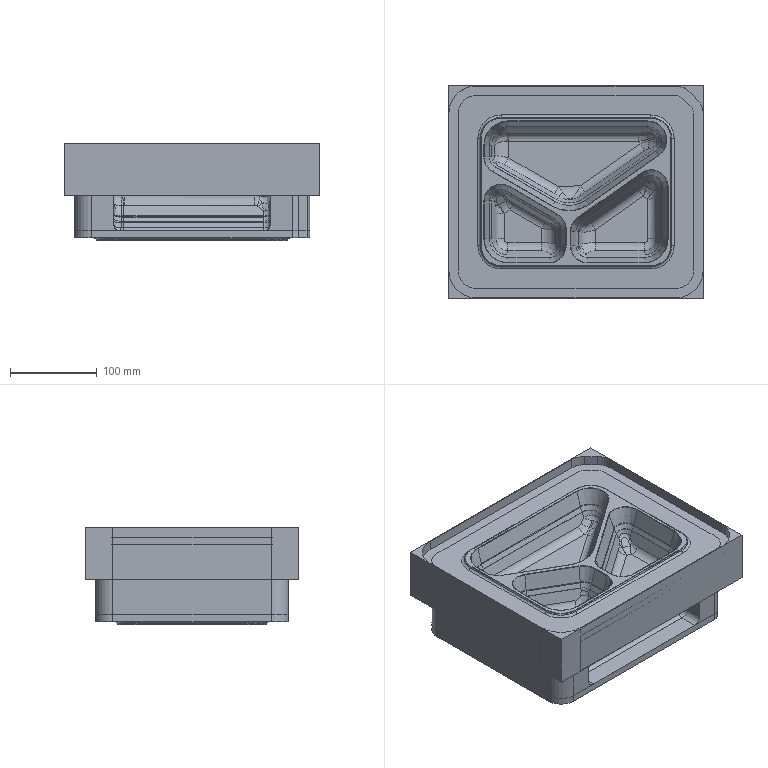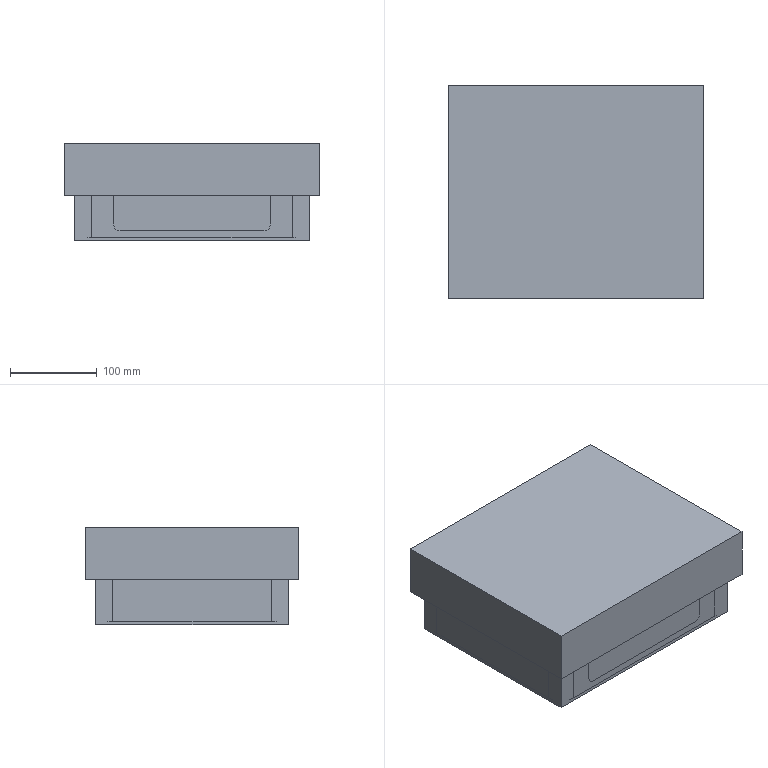CAM job | NX | 3-axis milling, drilling | part box 295.651 x 246.652 x 112.895 mm | stock box 295.651 x 246.652 x 112.895 mm
Tools:
number,name,description,diameter,corner_radius,flute_length,length,flutes
0,V2.0,Drilling Tool,2.0,0.0,35.0,50.0,2
0,D10,No Description,10.0,0.0,20.0,60.0,2
0,D8,No Description,8.0,0.0,0.0,40.0,2
0,D16R0.8,No Description,16.0,0.8,50.0,90.0,2
0,R2,No Description,4.0,2.0,0.0,20.0,2
Operations:
program,operation,operation_type,tool,method,geometry_group,spindle_rpm,surface_speed,feed_per_tooth,feed_cut,feed_plunge,cut_length_mm,path_length_mm,cut_time_min,machine_time_min
D-1,D1,CavityMilling,D16R0.8,METHOD,24D,7000.0,1099.0,0.3214,4500.0,100.0,378853.818,394407.122,84.19,85.745
D-2,D2,SurfaceContour,R2,METHOD,24D,8000.0,251.0,0.2812,4500.0,100.0,249101.044,250207.183,55.356,55.466
D-2,D3,Engraving,R2,METHOD,24D,9000.0,113.0,0.1111,2000.0,100.0,733.36,10181.661,0.7856,1.73
D-3,D4,Operation,V2.0,METHOD,24D,2000.0,75.0,0.0375,150.0,0.0,1285.0,6791.663,8.567,9.117
D-4,D5,FaceMilling,D10,METHOD,24D,7000.0,1099.0,0.2857,4000.0,100.0,4720.512,5040.744,1.18,1.212
D-4,D6,PlanarMilling,D10,METHOD,24D,7000.0,571.0,0.2857,4000.0,100.0,57884.32,58254.206,14.471,14.508
E-1,CAVITY_MILL_2,CavityMilling,D16R0.8,METHOD,24D_COPY,7000.0,1099.0,0.3214,4500.0,100.0,171576.372,175203.834,38.128,38.491
E-2,CAVITY_MILL_2_COPY,CavityMilling,D16R0.8,METHOD,24D_COPY_COPY,7000.0,1099.0,0.3214,4500.0,100.0,250337.681,254974.851,55.631,56.094
E-3,PLANAR_PROFILE,PlanarMilling,D8,METHOD,24D_COPY_COPY,8000.0,201.0,0.25,4000.0,100.0,19509.271,19857.271,4.877,4.912
E-3,PLANAR_PROFILE_COPY,PlanarMilling,D8,METHOD,24D_COPY_COPY,8000.0,201.0,0.25,4000.0,100.0,4818.268,5166.268,1.205,1.239